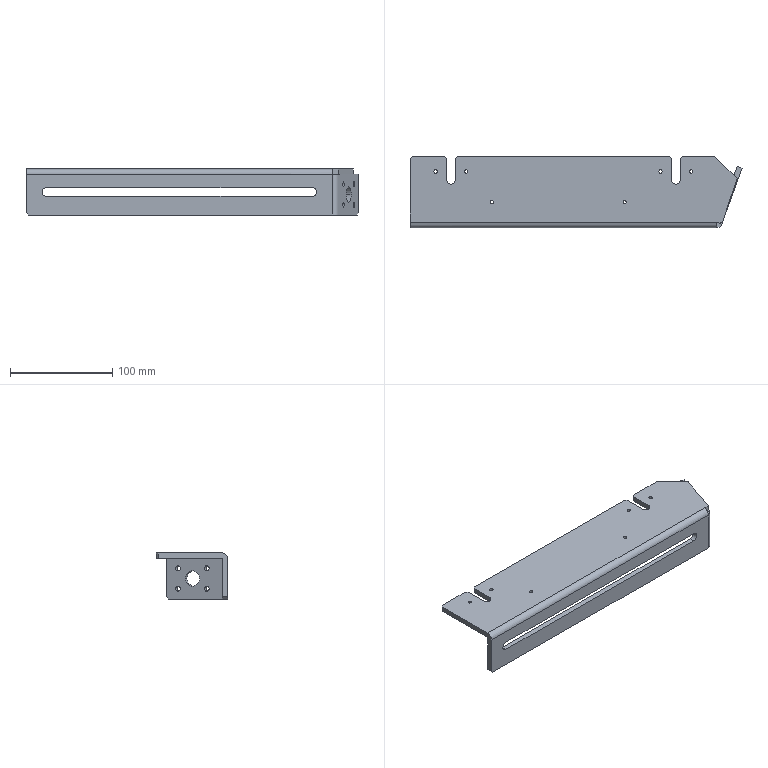Part | SolidWorks | features BaseBody 1 | 1 solid | 62 faces | box 324.706 x 70 x 45 mm | volume 163841 mm3 | plane 31 | cylinder 30 | spline 1 | commonest cylinder face diameters 3.3 x12 5 x8 8.5 x4 1 x2 11 x2 15 x2